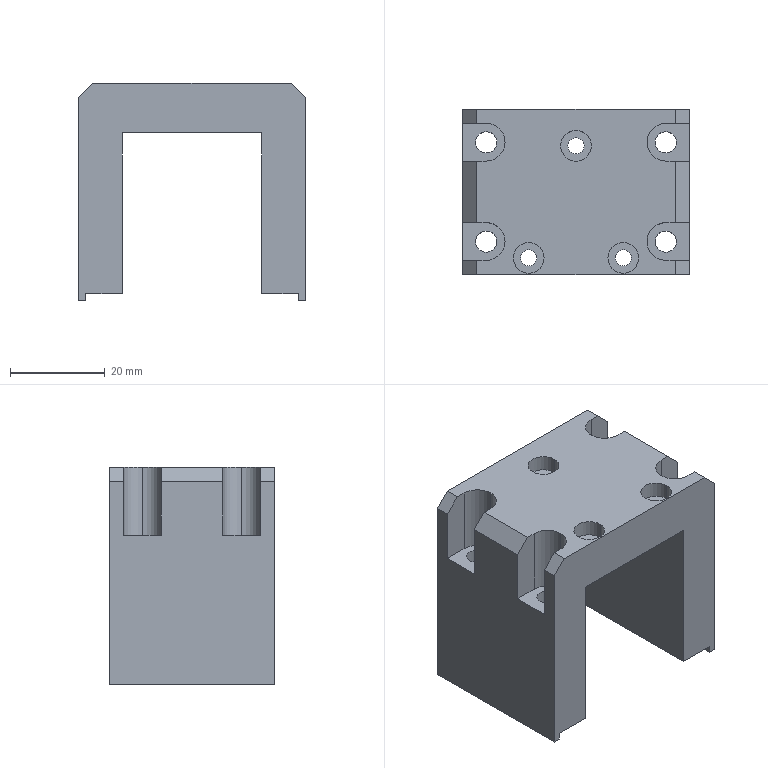Part | STEP file | 11-FG-S00611 | 1 solid | 61 faces | box 48 x 35 x 46 mm | volume 33562 mm3 | plane 35 | cylinder 26 | commonest cylinder face diameters 4.5 x8 3.4 x6 6.5 x6 8 x6